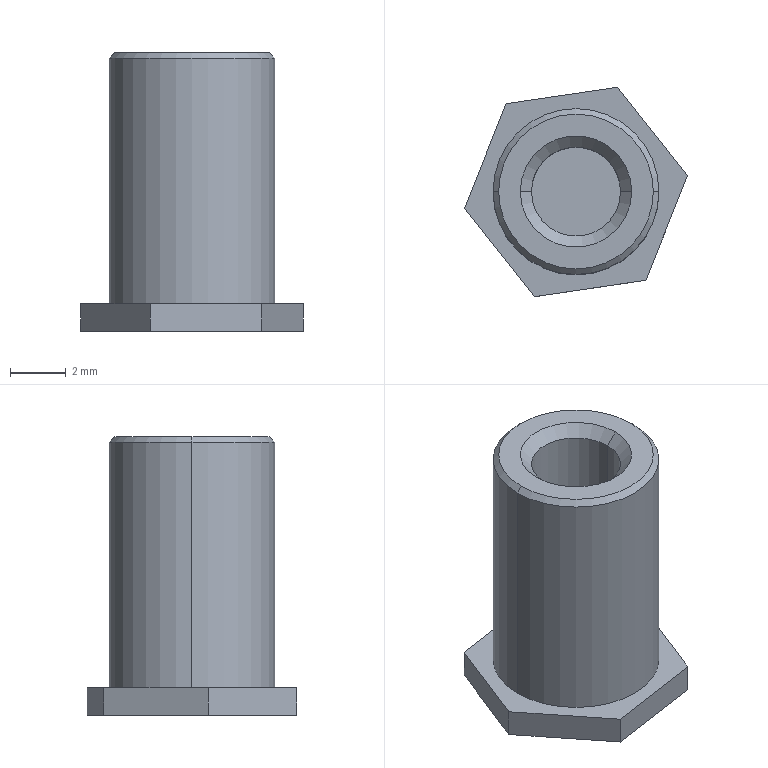Part | NX | features BREP 1 | 1 solid | 18 faces | box 7.997 x 7.514 x 10 mm | volume 235.147 mm3 | plane 10 | cylinder 4 | cone 4 | commonest cylinder face diameters 3.2 x2 5.95 x2
STEP:
#1=CARTESIAN_POINT('',(436.285,270.,18.8));
#2=VERTEX_POINT('',#1);
#3=CARTESIAN_POINT('',(442.235,270.,18.8));
#4=VERTEX_POINT('',#3);
#5=CARTESIAN_POINT('',(439.26,270.,18.8));
#6=DIRECTION('',(0.,0.,-1.));
#7=DIRECTION('',(-1.,0.,0.));
#8=AXIS2_PLACEMENT_3D('',#5,#6,#7);
#9=CIRCLE('',#8,2.975);
#10=EDGE_CURVE('',#2,#4,#9,.T.);
#11=ORIENTED_EDGE('',*,*,#10,.T.);
#12=CARTESIAN_POINT('',(442.235,270.,10.));
#13=VERTEX_POINT('',#12);
#14=CARTESIAN_POINT('',(442.235,270.,19.));
#15=DIRECTION('',(0.,0.,-1.));
#16=VECTOR('',#15,1000.);
#17=LINE('',#14,#16);
#18=EDGE_CURVE('',#13,#4,#17,.F.);
#19=ORIENTED_EDGE('',*,*,#18,.F.);
#20=CARTESIAN_POINT('',(436.285,270.,10.));
#21=VERTEX_POINT('',#20);
#22=CARTESIAN_POINT('',(439.26,270.,10.));
#23=DIRECTION('',(0.,0.,1.));
#24=DIRECTION('',(-1.,0.,0.));
#25=AXIS2_PLACEMENT_3D('',#22,#23,#24);
#26=CIRCLE('',#25,2.975);
#27=EDGE_CURVE('',#13,#21,#26,.T.);
#28=ORIENTED_EDGE('',*,*,#27,.T.);
#29=CARTESIAN_POINT('',(436.285,270.,19.));
#30=DIRECTION('',(0.,0.,-1.));
#31=VECTOR('',#30,1000.);
#32=LINE('',#29,#31);
#33=EDGE_CURVE('',#21,#2,#32,.F.);
#34=ORIENTED_EDGE('',*,*,#33,.T.);
#35=EDGE_LOOP('',(#11,#19,#28,#34));
#36=FACE_BOUND('',#35,.T.);
#37=CARTESIAN_POINT('',(439.26,270.,19.));
#38=DIRECTION('',(0.,0.,-1.));
#39=DIRECTION('',(1.,0.,0.));
#40=AXIS2_PLACEMENT_3D('',#37,#38,#39);
#41=CYLINDRICAL_SURFACE('',#40,2.975);
#42=ADVANCED_FACE('',(#36),#41,.T.);
#43=CARTESIAN_POINT('',(436.485,270.,19.));
#44=VERTEX_POINT('',#43);
#45=CARTESIAN_POINT('',(442.035,270.,19.));
#46=VERTEX_POINT('',#45);
#47=CARTESIAN_POINT('',(439.26,270.,19.));
#48=DIRECTION('',(0.,0.,-1.));
#49=DIRECTION('',(-1.,0.,0.));
#50=AXIS2_PLACEMENT_3D('',#47,#48,#49);
#51=CIRCLE('',#50,2.775);
#52=EDGE_CURVE('',#44,#46,#51,.T.);
#53=ORIENTED_EDGE('',*,*,#52,.T.);
#54=CARTESIAN_POINT('',(442.235,270.,18.8));
#55=DIRECTION('',(0.7071,0.,-0.7071));
#56=VECTOR('',#55,1000.);
#57=LINE('',#54,#56);
#58=EDGE_CURVE('',#4,#46,#57,.F.);
#59=ORIENTED_EDGE('',*,*,#58,.F.);
#60=ORIENTED_EDGE('',*,*,#10,.F.);
#61=CARTESIAN_POINT('',(436.285,270.,18.8));
#62=DIRECTION('',(-0.7071,0.,-0.7071));
#63=VECTOR('',#62,1000.);
#64=LINE('',#61,#63);
#65=EDGE_CURVE('',#2,#44,#64,.F.);
#66=ORIENTED_EDGE('',*,*,#65,.T.);
#67=EDGE_LOOP('',(#53,#59,#60,#66));
#68=FACE_BOUND('',#67,.T.);
#69=CARTESIAN_POINT('',(439.26,270.,18.8));
#70=DIRECTION('',(0.,0.,-1.));
#71=DIRECTION('',(1.,0.,0.));
#72=AXIS2_PLACEMENT_3D('',#69,#70,#71);
#73=CONICAL_SURFACE('',#72,2.975,0.7854);
#74=ADVANCED_FACE('',(#68),#73,.T.);
#75=CARTESIAN_POINT('',(437.66,270.,18.6));
#76=VERTEX_POINT('',#75);
#77=CARTESIAN_POINT('',(440.86,270.,18.6));
#78=VERTEX_POINT('',#77);
#79=CARTESIAN_POINT('',(439.26,270.,18.6));
#80=DIRECTION('',(0.,0.,1.));
#81=DIRECTION('',(1.,0.,0.));
#82=AXIS2_PLACEMENT_3D('',#79,#80,#81);
#83=CIRCLE('',#82,1.6);
#84=EDGE_CURVE('',#76,#78,#83,.T.);
#85=ORIENTED_EDGE('',*,*,#84,.F.);
#86=CARTESIAN_POINT('',(437.26,270.,19.));
#87=VERTEX_POINT('',#86);
#88=CARTESIAN_POINT('',(437.26,270.,19.));
#89=DIRECTION('',(-0.7071,0.,0.7071));
#90=VECTOR('',#89,1000.);
#91=LINE('',#88,#90);
#92=EDGE_CURVE('',#76,#87,#91,.T.);
#93=ORIENTED_EDGE('',*,*,#92,.T.);
#94=CARTESIAN_POINT('',(441.26,270.,19.));
#95=VERTEX_POINT('',#94);
#96=CARTESIAN_POINT('',(439.26,270.,19.));
#97=DIRECTION('',(0.,0.,-1.));
#98=DIRECTION('',(1.,0.,0.));
#99=AXIS2_PLACEMENT_3D('',#96,#97,#98);
#100=CIRCLE('',#99,2.);
#101=EDGE_CURVE('',#95,#87,#100,.T.);
#102=ORIENTED_EDGE('',*,*,#101,.F.);
#103=CARTESIAN_POINT('',(441.26,270.,19.));
#104=DIRECTION('',(0.7071,0.,0.7071));
#105=VECTOR('',#104,1000.);
#106=LINE('',#103,#105);
#107=EDGE_CURVE('',#78,#95,#106,.T.);
#108=ORIENTED_EDGE('',*,*,#107,.F.);
#109=EDGE_LOOP('',(#85,#93,#102,#108));
#110=FACE_BOUND('',#109,.T.);
#111=CARTESIAN_POINT('',(439.26,270.,19.));
#112=DIRECTION('',(0.,0.,1.));
#113=DIRECTION('',(-1.,0.,0.));
#114=AXIS2_PLACEMENT_3D('',#111,#112,#113);
#115=CONICAL_SURFACE('',#114,2.,0.7854);
#116=ADVANCED_FACE('',(#110),#115,.F.);
#117=CARTESIAN_POINT('',(437.66,270.,12.));
#118=VERTEX_POINT('',#117);
#119=CARTESIAN_POINT('',(440.86,270.,12.));
#120=VERTEX_POINT('',#119);
#121=CARTESIAN_POINT('',(439.26,270.,12.));
#122=DIRECTION('',(0.,0.,1.));
#123=DIRECTION('',(1.,0.,0.));
#124=AXIS2_PLACEMENT_3D('',#121,#122,#123);
#125=CIRCLE('',#124,1.6);
#126=EDGE_CURVE('',#118,#120,#125,.T.);
#127=ORIENTED_EDGE('',*,*,#126,.F.);
#128=CARTESIAN_POINT('',(437.66,270.,12.));
#129=DIRECTION('',(0.,0.,1.));
#130=VECTOR('',#129,1000.);
#131=LINE('',#128,#130);
#132=EDGE_CURVE('',#118,#76,#131,.T.);
#133=ORIENTED_EDGE('',*,*,#132,.T.);
#134=ORIENTED_EDGE('',*,*,#84,.T.);
#135=CARTESIAN_POINT('',(440.86,270.,12.));
#136=DIRECTION('',(0.,0.,1.));
#137=VECTOR('',#136,1000.);
#138=LINE('',#135,#137);
#139=EDGE_CURVE('',#120,#78,#138,.T.);
#140=ORIENTED_EDGE('',*,*,#139,.F.);
#141=EDGE_LOOP('',(#127,#133,#134,#140));
#142=FACE_BOUND('',#141,.T.);
#143=CARTESIAN_POINT('',(439.26,270.,12.));
#144=DIRECTION('',(0.,0.,1.));
#145=DIRECTION('',(-1.,0.,0.));
#146=AXIS2_PLACEMENT_3D('',#143,#144,#145);
#147=CYLINDRICAL_SURFACE('',#146,1.6);
#148=ADVANCED_FACE('',(#142),#147,.F.);
#149=ORIENTED_EDGE('',*,*,#18,.T.);
#150=CARTESIAN_POINT('',(439.26,270.,18.8));
#151=DIRECTION('',(0.,0.,-1.));
#152=DIRECTION('',(-1.,0.,0.));
#153=AXIS2_PLACEMENT_3D('',#150,#151,#152);
#154=CIRCLE('',#153,2.975);
#155=EDGE_CURVE('',#4,#2,#154,.T.);
#156=ORIENTED_EDGE('',*,*,#155,.T.);
#157=ORIENTED_EDGE('',*,*,#33,.F.);
#158=CARTESIAN_POINT('',(439.26,270.,10.));
#159=DIRECTION('',(0.,0.,1.));
#160=DIRECTION('',(-1.,0.,0.));
#161=AXIS2_PLACEMENT_3D('',#158,#159,#160);
#162=CIRCLE('',#161,2.975);
#163=EDGE_CURVE('',#21,#13,#162,.T.);
#164=ORIENTED_EDGE('',*,*,#163,.T.);
#165=EDGE_LOOP('',(#149,#156,#157,#164));
#166=FACE_BOUND('',#165,.T.);
#167=CARTESIAN_POINT('',(439.26,270.,19.));
#168=DIRECTION('',(0.,0.,-1.));
#169=DIRECTION('',(1.,0.,0.));
#170=AXIS2_PLACEMENT_3D('',#167,#168,#169);
#171=CYLINDRICAL_SURFACE('',#170,2.975);
#172=ADVANCED_FACE('',(#166),#171,.T.);
#173=CARTESIAN_POINT('',(435.262,269.411,10.));
#174=VERTEX_POINT('',#173);
#175=CARTESIAN_POINT('',(437.771,266.243,10.));
#176=VERTEX_POINT('',#175);
#177=CARTESIAN_POINT('',(435.262,269.411,10.));
#178=DIRECTION('',(0.6209,-0.7839,0.));
#179=VECTOR('',#178,1000.);
#180=LINE('',#177,#179);
#181=EDGE_CURVE('',#174,#176,#180,.T.);
#182=ORIENTED_EDGE('',*,*,#181,.T.);
#183=CARTESIAN_POINT('',(441.769,266.832,10.));
#184=VERTEX_POINT('',#183);
#185=CARTESIAN_POINT('',(437.771,266.243,10.));
#186=DIRECTION('',(0.9893,0.1457,0.));
#187=VECTOR('',#186,1000.);
#188=LINE('',#185,#187);
#189=EDGE_CURVE('',#176,#184,#188,.T.);
#190=ORIENTED_EDGE('',*,*,#189,.T.);
#191=CARTESIAN_POINT('',(443.258,270.589,10.));
#192=VERTEX_POINT('',#191);
#193=CARTESIAN_POINT('',(441.769,266.832,10.));
#194=DIRECTION('',(0.3684,0.9297,0.));
#195=VECTOR('',#194,1000.);
#196=LINE('',#193,#195);
#197=EDGE_CURVE('',#184,#192,#196,.T.);
#198=ORIENTED_EDGE('',*,*,#197,.T.);
#199=CARTESIAN_POINT('',(440.749,273.757,10.));
#200=VERTEX_POINT('',#199);
#201=CARTESIAN_POINT('',(443.258,270.589,10.));
#202=DIRECTION('',(-0.6209,0.7839,0.));
#203=VECTOR('',#202,1000.);
#204=LINE('',#201,#203);
#205=EDGE_CURVE('',#192,#200,#204,.T.);
#206=ORIENTED_EDGE('',*,*,#205,.T.);
#207=CARTESIAN_POINT('',(436.751,273.168,10.));
#208=VERTEX_POINT('',#207);
#209=CARTESIAN_POINT('',(440.749,273.757,10.));
#210=DIRECTION('',(-0.9893,-0.1457,0.));
#211=VECTOR('',#210,1000.);
#212=LINE('',#209,#211);
#213=EDGE_CURVE('',#200,#208,#212,.T.);
#214=ORIENTED_EDGE('',*,*,#213,.T.);
#215=CARTESIAN_POINT('',(436.751,273.168,10.));
#216=DIRECTION('',(-0.3684,-0.9297,0.));
#217=VECTOR('',#216,1000.);
#218=LINE('',#215,#217);
#219=EDGE_CURVE('',#208,#174,#218,.T.);
#220=ORIENTED_EDGE('',*,*,#219,.T.);
#221=EDGE_LOOP('',(#182,#190,#198,#206,#214,#220));
#222=FACE_BOUND('',#221,.T.);
#223=ORIENTED_EDGE('',*,*,#163,.F.);
#224=ORIENTED_EDGE('',*,*,#27,.F.);
#225=EDGE_LOOP('',(#223,#224));
#226=FACE_BOUND('',#225,.T.);
#227=CARTESIAN_POINT('',(439.26,270.,10.));
#228=DIRECTION('',(0.,0.,1.));
#229=DIRECTION('',(-1.,0.,0.));
#230=AXIS2_PLACEMENT_3D('',#227,#228,#229);
#231=PLANE('',#230);
#232=ADVANCED_FACE('',(#222,#226),#231,.T.);
#233=ORIENTED_EDGE('',*,*,#58,.T.);
#234=CARTESIAN_POINT('',(439.26,270.,19.));
#235=DIRECTION('',(0.,0.,-1.));
#236=DIRECTION('',(-1.,0.,0.));
#237=AXIS2_PLACEMENT_3D('',#234,#235,#236);
#238=CIRCLE('',#237,2.775);
#239=EDGE_CURVE('',#46,#44,#238,.T.);
#240=ORIENTED_EDGE('',*,*,#239,.T.);
#241=ORIENTED_EDGE('',*,*,#65,.F.);
#242=ORIENTED_EDGE('',*,*,#155,.F.);
#243=EDGE_LOOP('',(#233,#240,#241,#242));
#244=FACE_BOUND('',#243,.T.);
#245=CARTESIAN_POINT('',(439.26,270.,18.8));
#246=DIRECTION('',(0.,0.,-1.));
#247=DIRECTION('',(1.,0.,0.));
#248=AXIS2_PLACEMENT_3D('',#245,#246,#247);
#249=CONICAL_SURFACE('',#248,2.975,0.7854);
#250=ADVANCED_FACE('',(#244),#249,.T.);
#251=CARTESIAN_POINT('',(441.769,266.832,9.));
#252=VERTEX_POINT('',#251);
#253=CARTESIAN_POINT('',(437.771,266.243,9.));
#254=VERTEX_POINT('',#253);
#255=CARTESIAN_POINT('',(437.771,266.243,9.));
#256=DIRECTION('',(-0.9893,-0.1457,0.));
#257=VECTOR('',#256,1000.);
#258=LINE('',#255,#257);
#259=EDGE_CURVE('',#252,#254,#258,.T.);
#260=ORIENTED_EDGE('',*,*,#259,.F.);
#261=CARTESIAN_POINT('',(441.769,266.832,10.));
#262=DIRECTION('',(0.,0.,-1.));
#263=VECTOR('',#262,1000.);
#264=LINE('',#261,#263);
#265=EDGE_CURVE('',#184,#252,#264,.T.);
#266=ORIENTED_EDGE('',*,*,#265,.F.);
#267=ORIENTED_EDGE('',*,*,#189,.F.);
#268=CARTESIAN_POINT('',(437.771,266.243,10.));
#269=DIRECTION('',(0.,0.,1.));
#270=VECTOR('',#269,1000.);
#271=LINE('',#268,#270);
#272=EDGE_CURVE('',#254,#176,#271,.T.);
#273=ORIENTED_EDGE('',*,*,#272,.F.);
#274=EDGE_LOOP('',(#260,#266,#267,#273));
#275=FACE_BOUND('',#274,.T.);
#276=CARTESIAN_POINT('',(437.771,266.243,10.));
#277=DIRECTION('',(-0.1457,0.9893,0.));
#278=DIRECTION('',(0.9893,0.1457,0.));
#279=AXIS2_PLACEMENT_3D('',#276,#277,#278);
#280=PLANE('',#279);
#281=ADVANCED_FACE('',(#275),#280,.F.);
#282=CARTESIAN_POINT('',(435.262,269.411,9.));
#283=VERTEX_POINT('',#282);
#284=CARTESIAN_POINT('',(435.262,269.411,9.));
#285=DIRECTION('',(-0.6209,0.7839,0.));
#286=VECTOR('',#285,1000.);
#287=LINE('',#284,#286);
#288=EDGE_CURVE('',#254,#283,#287,.T.);
#289=ORIENTED_EDGE('',*,*,#288,.F.);
#290=ORIENTED_EDGE('',*,*,#272,.T.);
#291=ORIENTED_EDGE('',*,*,#181,.F.);
#292=CARTESIAN_POINT('',(435.262,269.411,10.));
#293=DIRECTION('',(0.,0.,1.));
#294=VECTOR('',#293,1000.);
#295=LINE('',#292,#294);
#296=EDGE_CURVE('',#283,#174,#295,.T.);
#297=ORIENTED_EDGE('',*,*,#296,.F.);
#298=EDGE_LOOP('',(#289,#290,#291,#297));
#299=FACE_BOUND('',#298,.T.);
#300=CARTESIAN_POINT('',(435.262,269.411,10.));
#301=DIRECTION('',(0.7839,0.6209,0.));
#302=DIRECTION('',(0.6209,-0.7839,0.));
#303=AXIS2_PLACEMENT_3D('',#300,#301,#302);
#304=PLANE('',#303);
#305=ADVANCED_FACE('',(#299),#304,.F.);
#306=CARTESIAN_POINT('',(436.751,273.168,9.));
#307=VERTEX_POINT('',#306);
#308=CARTESIAN_POINT('',(436.751,273.168,9.));
#309=DIRECTION('',(0.3684,0.9297,0.));
#310=VECTOR('',#309,1000.);
#311=LINE('',#308,#310);
#312=EDGE_CURVE('',#283,#307,#311,.T.);
#313=ORIENTED_EDGE('',*,*,#312,.F.);
#314=ORIENTED_EDGE('',*,*,#296,.T.);
#315=ORIENTED_EDGE('',*,*,#219,.F.);
#316=CARTESIAN_POINT('',(436.751,273.168,10.));
#317=DIRECTION('',(0.,0.,1.));
#318=VECTOR('',#317,1000.);
#319=LINE('',#316,#318);
#320=EDGE_CURVE('',#307,#208,#319,.T.);
#321=ORIENTED_EDGE('',*,*,#320,.F.);
#322=EDGE_LOOP('',(#313,#314,#315,#321));
#323=FACE_BOUND('',#322,.T.);
#324=CARTESIAN_POINT('',(436.751,273.168,10.));
#325=DIRECTION('',(0.9297,-0.3684,0.));
#326=DIRECTION('',(-0.3684,-0.9297,0.));
#327=AXIS2_PLACEMENT_3D('',#324,#325,#326);
#328=PLANE('',#327);
#329=ADVANCED_FACE('',(#323),#328,.F.);
#330=CARTESIAN_POINT('',(440.749,273.757,9.));
#331=VERTEX_POINT('',#330);
#332=CARTESIAN_POINT('',(440.749,273.757,9.));
#333=DIRECTION('',(0.9893,0.1457,0.));
#334=VECTOR('',#333,1000.);
#335=LINE('',#332,#334);
#336=EDGE_CURVE('',#307,#331,#335,.T.);
#337=ORIENTED_EDGE('',*,*,#336,.F.);
#338=ORIENTED_EDGE('',*,*,#320,.T.);
#339=ORIENTED_EDGE('',*,*,#213,.F.);
#340=CARTESIAN_POINT('',(440.749,273.757,10.));
#341=DIRECTION('',(0.,0.,1.));
#342=VECTOR('',#341,1000.);
#343=LINE('',#340,#342);
#344=EDGE_CURVE('',#331,#200,#343,.T.);
#345=ORIENTED_EDGE('',*,*,#344,.F.);
#346=EDGE_LOOP('',(#337,#338,#339,#345));
#347=FACE_BOUND('',#346,.T.);
#348=CARTESIAN_POINT('',(440.749,273.757,10.));
#349=DIRECTION('',(0.1457,-0.9893,0.));
#350=DIRECTION('',(-0.9893,-0.1457,0.));
#351=AXIS2_PLACEMENT_3D('',#348,#349,#350);
#352=PLANE('',#351);
#353=ADVANCED_FACE('',(#347),#352,.F.);
#354=CARTESIAN_POINT('',(443.258,270.589,9.));
#355=VERTEX_POINT('',#354);
#356=CARTESIAN_POINT('',(443.258,270.589,9.));
#357=DIRECTION('',(0.6209,-0.7839,0.));
#358=VECTOR('',#357,1000.);
#359=LINE('',#356,#358);
#360=EDGE_CURVE('',#331,#355,#359,.T.);
#361=ORIENTED_EDGE('',*,*,#360,.F.);
#362=ORIENTED_EDGE('',*,*,#344,.T.);
#363=ORIENTED_EDGE('',*,*,#205,.F.);
#364=CARTESIAN_POINT('',(443.258,270.589,10.));
#365=DIRECTION('',(0.,0.,1.));
#366=VECTOR('',#365,1000.);
#367=LINE('',#364,#366);
#368=EDGE_CURVE('',#355,#192,#367,.T.);
#369=ORIENTED_EDGE('',*,*,#368,.F.);
#370=EDGE_LOOP('',(#361,#362,#363,#369));
#371=FACE_BOUND('',#370,.T.);
#372=CARTESIAN_POINT('',(443.258,270.589,10.));
#373=DIRECTION('',(-0.7839,-0.6209,0.));
#374=DIRECTION('',(-0.6209,0.7839,0.));
#375=AXIS2_PLACEMENT_3D('',#372,#373,#374);
#376=PLANE('',#375);
#377=ADVANCED_FACE('',(#371),#376,.F.);
#378=CARTESIAN_POINT('',(441.769,266.832,9.));
#379=DIRECTION('',(-0.3684,-0.9297,0.));
#380=VECTOR('',#379,1000.);
#381=LINE('',#378,#380);
#382=EDGE_CURVE('',#355,#252,#381,.T.);
#383=ORIENTED_EDGE('',*,*,#382,.F.);
#384=ORIENTED_EDGE('',*,*,#368,.T.);
#385=ORIENTED_EDGE('',*,*,#197,.F.);
#386=ORIENTED_EDGE('',*,*,#265,.T.);
#387=EDGE_LOOP('',(#383,#384,#385,#386));
#388=FACE_BOUND('',#387,.T.);
#389=CARTESIAN_POINT('',(441.769,266.832,10.));
#390=DIRECTION('',(-0.9297,0.3684,0.));
#391=DIRECTION('',(0.3684,0.9297,0.));
#392=AXIS2_PLACEMENT_3D('',#389,#390,#391);
#393=PLANE('',#392);
#394=ADVANCED_FACE('',(#388),#393,.F.);
#395=ORIENTED_EDGE('',*,*,#52,.F.);
#396=ORIENTED_EDGE('',*,*,#239,.F.);
#397=EDGE_LOOP('',(#395,#396));
#398=FACE_BOUND('',#397,.T.);
#399=ORIENTED_EDGE('',*,*,#101,.T.);
#400=CARTESIAN_POINT('',(439.26,270.,19.));
#401=DIRECTION('',(0.,0.,-1.));
#402=DIRECTION('',(1.,0.,0.));
#403=AXIS2_PLACEMENT_3D('',#400,#401,#402);
#404=CIRCLE('',#403,2.);
#405=EDGE_CURVE('',#87,#95,#404,.T.);
#406=ORIENTED_EDGE('',*,*,#405,.T.);
#407=EDGE_LOOP('',(#399,#406));
#408=FACE_BOUND('',#407,.T.);
#409=CARTESIAN_POINT('',(439.26,270.,19.));
#410=DIRECTION('',(0.,0.,1.));
#411=DIRECTION('',(-1.,0.,0.));
#412=AXIS2_PLACEMENT_3D('',#409,#410,#411);
#413=PLANE('',#412);
#414=ADVANCED_FACE('',(#398,#408),#413,.T.);
#415=ORIENTED_EDGE('',*,*,#382,.T.);
#416=ORIENTED_EDGE('',*,*,#259,.T.);
#417=ORIENTED_EDGE('',*,*,#288,.T.);
#418=ORIENTED_EDGE('',*,*,#312,.T.);
#419=ORIENTED_EDGE('',*,*,#336,.T.);
#420=ORIENTED_EDGE('',*,*,#360,.T.);
#421=EDGE_LOOP('',(#415,#416,#417,#418,#419,#420));
#422=FACE_BOUND('',#421,.T.);
#423=CARTESIAN_POINT('',(439.26,270.,9.));
#424=DIRECTION('',(0.,0.,1.));
#425=DIRECTION('',(-1.,0.,0.));
#426=AXIS2_PLACEMENT_3D('',#423,#424,#425);
#427=PLANE('',#426);
#428=ADVANCED_FACE('',(#422),#427,.F.);
#429=ORIENTED_EDGE('',*,*,#92,.F.);
#430=CARTESIAN_POINT('',(439.26,270.,18.6));
#431=DIRECTION('',(0.,0.,1.));
#432=DIRECTION('',(1.,0.,0.));
#433=AXIS2_PLACEMENT_3D('',#430,#431,#432);
#434=CIRCLE('',#433,1.6);
#435=EDGE_CURVE('',#78,#76,#434,.T.);
#436=ORIENTED_EDGE('',*,*,#435,.F.);
#437=ORIENTED_EDGE('',*,*,#107,.T.);
#438=ORIENTED_EDGE('',*,*,#405,.F.);
#439=EDGE_LOOP('',(#429,#436,#437,#438));
#440=FACE_BOUND('',#439,.T.);
#441=CARTESIAN_POINT('',(439.26,270.,19.));
#442=DIRECTION('',(0.,0.,1.));
#443=DIRECTION('',(-1.,0.,0.));
#444=AXIS2_PLACEMENT_3D('',#441,#442,#443);
#445=CONICAL_SURFACE('',#444,2.,0.7854);
#446=ADVANCED_FACE('',(#440),#445,.F.);
#447=ORIENTED_EDGE('',*,*,#132,.F.);
#448=CARTESIAN_POINT('',(439.26,270.,12.));
#449=DIRECTION('',(0.,0.,1.));
#450=DIRECTION('',(1.,0.,0.));
#451=AXIS2_PLACEMENT_3D('',#448,#449,#450);
#452=CIRCLE('',#451,1.6);
#453=EDGE_CURVE('',#120,#118,#452,.T.);
#454=ORIENTED_EDGE('',*,*,#453,.F.);
#455=ORIENTED_EDGE('',*,*,#139,.T.);
#456=ORIENTED_EDGE('',*,*,#435,.T.);
#457=EDGE_LOOP('',(#447,#454,#455,#456));
#458=FACE_BOUND('',#457,.T.);
#459=CARTESIAN_POINT('',(439.26,270.,12.));
#460=DIRECTION('',(0.,0.,1.));
#461=DIRECTION('',(-1.,0.,0.));
#462=AXIS2_PLACEMENT_3D('',#459,#460,#461);
#463=CYLINDRICAL_SURFACE('',#462,1.6);
#464=ADVANCED_FACE('',(#458),#463,.F.);
#465=ORIENTED_EDGE('',*,*,#453,.T.);
#466=ORIENTED_EDGE('',*,*,#126,.T.);
#467=EDGE_LOOP('',(#465,#466));
#468=FACE_BOUND('',#467,.T.);
#469=CARTESIAN_POINT('',(439.26,270.,12.));
#470=DIRECTION('',(0.,0.,1.));
#471=DIRECTION('',(-1.,0.,0.));
#472=AXIS2_PLACEMENT_3D('',#469,#470,#471);
#473=PLANE('',#472);
#474=ADVANCED_FACE('',(#468),#473,.T.);
#475=CLOSED_SHELL('',(#42,#74,#116,#148,#172,#232,#250,#281,#305,#329,#353,#377,#394,#414,#428,#446,#464,#474));
#476=MANIFOLD_SOLID_BREP('',#475);
#477=(LENGTH_UNIT()NAMED_UNIT(*)SI_UNIT(.MILLI.,.METRE.));
#478=UNCERTAINTY_MEASURE_WITH_UNIT(LENGTH_MEASURE(0.00001),#477,'','');
#479=(NAMED_UNIT(*)PLANE_ANGLE_UNIT()SI_UNIT($,.RADIAN.));
#480=(NAMED_UNIT(*)SI_UNIT($,.STERADIAN.)SOLID_ANGLE_UNIT());
#481=(GEOMETRIC_REPRESENTATION_CONTEXT(3)GLOBAL_UNCERTAINTY_ASSIGNED_CONTEXT((#478))GLOBAL_UNIT_ASSIGNED_CONTEXT((#477,#479,#480))REPRESENTATION_CONTEXT('',''));
#482=ADVANCED_BREP_SHAPE_REPRESENTATION('',(#476),#481);